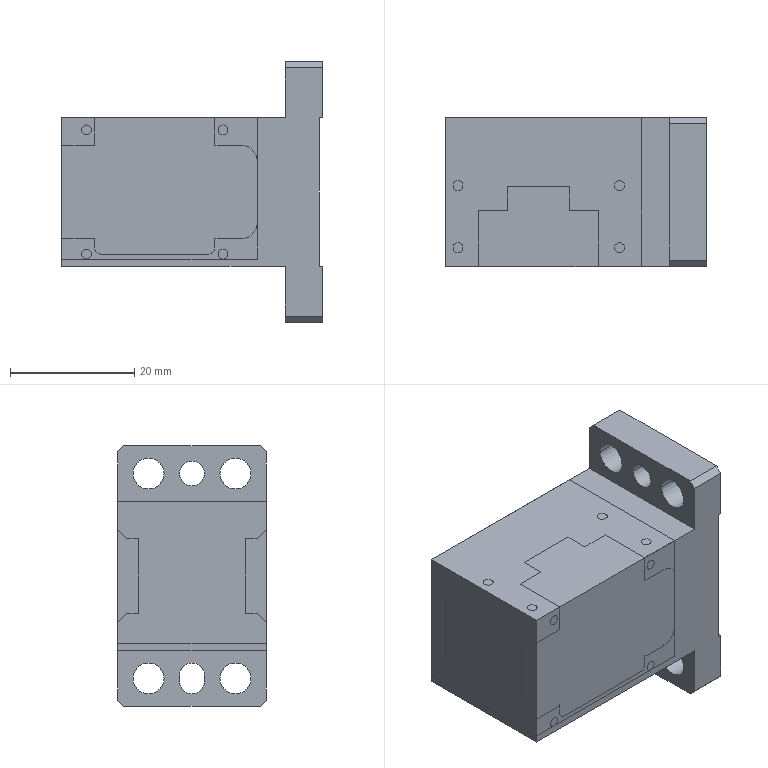NC program | NX | posted with a generic post | part box 42 x 24 x 42 mm
Lines 8998 to 10020 of 31406:
(CAVITY_MILL_COPY , TOOL : D2)
N17982 T02 M6
N17984 G54
N17986 G17 G0 G90 X-3.449 Y9.065 B0. C0. S6500 M3
N17988 G43 Z30. H2
N17990 Z0.465
N17992 G94 G1 Z-0.035 F1000.
N17994 G3 X-4.249 Y9.465 R1.
N17996 G1 X-5. F800.
N17998 G3 X-6.465 Y8. R1.465
N18000 G1 Y7.249
N18002 G3 X-6.065 Y6.449 R1.
N18004 G1 Z0.465
N18006 G0 X-3.414 Y9.03 Z0.43
N18008 G1 Z-0.07 F1000.
N18010 G3 X-4.214 Y9.43 R1.
N18012 G1 X-5. F800.
N18014 G3 X-6.43 Y8. R1.43
N18016 G1 Y7.214
N18018 G3 X-6.03 Y6.414 R1.
N18020 G1 Z0.43
N18022 G0 X-3.379 Y8.995 Z0.395
N18024 G1 Z-0.105 F1000.
N18026 G3 X-4.179 Y9.395 R1.
N18028 G1 X-5. F800.
N18030 G3 X-6.395 Y8. R1.395
N18032 G1 Y7.179
N18034 G3 X-5.995 Y6.379 R1.
N18036 G1 Z0.395
N18038 G0 X-3.344 Y8.96 Z0.36
N18040 G1 Z-0.14 F1000.
N18042 G3 X-4.144 Y9.36 R1.
N18044 G1 X-5. F800.
N18046 G3 X-6.36 Y8. R1.36
N18048 G1 Y7.144
N18050 G3 X-5.96 Y6.344 R1.
N18052 G1 Z0.36
N18054 G0 X-3.309 Y8.925 Z0.325
N18056 G1 Z-0.175 F1000.
N18058 G3 X-4.109 Y9.325 R1.
N18060 G1 X-5. F800.
N18062 G3 X-6.325 Y8. R1.325
N18064 G1 Y7.109
N18066 G3 X-5.925 Y6.309 R1.
N18068 G1 Z0.325
N18070 G0 X-3.274 Y8.89 Z0.29
N18072 G1 Z-0.21 F1000.
N18074 G3 X-4.074 Y9.29 R1.
N18076 G1 X-5. F800.
N18078 G3 X-6.29 Y8. R1.29
N18080 G1 Y7.074
N18082 G3 X-5.89 Y6.274 R1.
N18084 G1 Z0.29
N18086 G0 X-3.239 Y8.855 Z0.255
N18088 G1 Z-0.245 F1000.
N18090 G3 X-4.039 Y9.255 R1.
N18092 G1 X-5. F800.
N18094 G3 X-6.255 Y8. R1.255
N18096 G1 Y7.039
N18098 G3 X-5.855 Y6.239 R1.
N18100 G1 Z0.255
N18102 G0 X-3.204 Y8.82 Z0.22
N18104 G1 Z-0.28 F1000.
N18106 G3 X-4.004 Y9.22 R1.
N18108 G1 X-5. F800.
N18110 G3 X-6.22 Y8. R1.22
N18112 G1 Y7.004
N18114 G3 X-5.82 Y6.204 R1.
N18116 G1 Z0.22
N18118 G0 X-3.169 Y8.785 Z0.185
N18120 G1 Z-0.315 F1000.
N18122 G3 X-3.969 Y9.185 R1.
N18124 G1 X-5. F800.
N18126 G3 X-6.185 Y8. R1.185
N18128 G1 Y6.969
N18130 G3 X-5.785 Y6.169 R1.
N18132 G1 Z0.185
N18134 G0 X-3.134 Y8.75 Z0.15
N18136 G1 Z-0.35 F1000.
N18138 G3 X-3.934 Y9.15 R1.
N18140 G1 X-5. F800.
N18142 G3 X-6.15 Y8. R1.15
N18144 G1 Y6.934
N18146 G3 X-5.75 Y6.134 R1.
N18148 G1 Z0.15
N18150 G0 X-3.099 Y8.715 Z0.115
N18152 G1 Z-0.385 F1000.
N18154 G3 X-3.899 Y9.115 R1.
N18156 G1 X-5. F800.
N18158 G3 X-6.115 Y8. R1.115
N18160 G1 Y6.899
N18162 G3 X-5.715 Y6.099 R1.
N18164 G1 Z0.115
N18166 G0 X-3.064 Y8.68 Z0.08
N18168 G1 Z-0.42 F1000.
N18170 G3 X-3.864 Y9.08 R1.
N18172 G1 X-5. F800.
N18174 G3 X-6.08 Y8. R1.08
N18176 G1 Y6.864
N18178 G3 X-5.68 Y6.064 R1.
N18180 G1 Z0.08
N18182 G0 X-3.029 Y8.645 Z0.045
N18184 G1 Z-0.455 F1000.
N18186 G3 X-3.829 Y9.045 R1.
N18188 G1 X-5. F800.
N18190 G3 X-6.045 Y8. R1.045
N18192 G1 Y6.829
N18194 G3 X-5.645 Y6.029 R1.
N18196 G1 Z0.045
N18198 G0 X-2.994 Y8.61 Z0.01
N18200 G1 Z-0.49 F1000.
N18202 G3 X-3.794 Y9.01 R1.
N18204 G1 X-5. F800.
N18206 G3 X-6.01 Y8. R1.01
N18208 G1 Y6.794
N18210 G3 X-5.61 Y5.994 R1.
N18212 G1 Z0.01
N18214 G0 X-2.959 Y8.575 Z-0.025
N18216 G1 Z-0.525 F1000.
N18218 G3 X-3.759 Y8.975 R1.
N18220 G1 X-5. F800.
N18222 G3 X-5.975 Y8. R0.975
N18224 G1 Y6.759
N18226 G3 X-5.575 Y5.959 R1.
N18228 G1 Z-0.025
N18230 G0 X-2.924 Y8.54 Z-0.06
N18232 G1 Z-0.56 F1000.
N18234 G3 X-3.724 Y8.94 R1.
N18236 G1 X-5. F800.
N18238 G3 X-5.94 Y8. R0.94
N18240 G1 Y6.724
N18242 G3 X-5.54 Y5.924 R1.
N18244 G1 Z-0.06
N18246 G0 X-2.889 Y8.505 Z-0.095
N18248 G1 Z-0.595 F1000.
N18250 G3 X-3.689 Y8.905 R1.
N18252 G1 X-5. F800.
N18254 G3 X-5.905 Y8. R0.905
N18256 G1 Y6.689
N18258 G3 X-5.505 Y5.889 R1.
N18260 G1 Z-0.095
N18262 G0 X-2.854 Y8.47 Z-0.13
N18264 G1 Z-0.63 F1000.
N18266 G3 X-3.654 Y8.87 R1.
N18268 G1 X-5. F800.
N18270 G3 X-5.87 Y8. R0.87
N18272 G1 Y6.654
N18274 G3 X-5.47 Y5.854 R1.
N18276 G1 Z-0.13
N18278 G0 X-2.819 Y8.435 Z-0.165
N18280 G1 Z-0.665 F1000.
N18282 G3 X-3.619 Y8.835 R1.
N18284 G1 X-5. F800.
N18286 G3 X-5.835 Y8. R0.835
N18288 G1 Y6.619
N18290 G3 X-5.435 Y5.819 R1.
N18292 G1 Z-0.165
N18294 G0 X-2.784 Y8.4 Z-0.2
N18296 G1 Z-0.7 F1000.
N18298 G3 X-3.584 Y8.8 R1.
N18300 G1 X-5. F800.
N18302 G3 X-5.8 Y8. R0.8
N18304 G1 Y6.584
N18306 G3 X-5.4 Y5.784 R1.
N18308 G1 Z-0.2
N18310 G0 X-2.749 Y8.365 Z-0.235
N18312 G1 Z-0.735 F1000.
N18314 G3 X-3.549 Y8.765 R1.
N18316 G1 X-5. F800.
N18318 G3 X-5.765 Y8. R0.765
N18320 G1 Y6.549
N18322 G3 X-5.365 Y5.749 R1.
N18324 G1 Z-0.235
N18326 G0 X-2.714 Y8.33 Z-0.27
N18328 G1 Z-0.77 F1000.
N18330 G3 X-3.514 Y8.73 R1.
N18332 G1 X-5. F800.
N18334 G3 X-5.73 Y8. R0.73
N18336 G1 Y6.514
N18338 G3 X-5.33 Y5.714 R1.
N18340 G1 Z-0.27
N18342 G0 X-2.679 Y8.295 Z-0.305
N18344 G1 Z-0.805 F1000.
N18346 G3 X-3.479 Y8.695 R1.
N18348 G1 X-5. F800.
N18350 G3 X-5.695 Y8. R0.695
N18352 G1 Y6.479
N18354 G3 X-5.295 Y5.679 R1.
N18356 G1 Z-0.305
N18358 G0 X-2.644 Y8.26 Z-0.34
N18360 G1 Z-0.84 F1000.
N18362 G3 X-3.444 Y8.66 R1.
N18364 G1 X-5. F800.
N18366 G3 X-5.66 Y8. R0.66
N18368 G1 Y6.444
N18370 G3 X-5.26 Y5.644 R1.
N18372 G1 Z-0.34
N18374 G0 X-2.609 Y8.225 Z-0.375
N18376 G1 Z-0.875 F1000.
N18378 G3 X-3.409 Y8.625 R1.
N18380 G1 X-5. F800.
N18382 G3 X-5.625 Y8. R0.625
N18384 G1 Y6.409
N18386 G3 X-5.225 Y5.609 R1.
N18388 G1 Z-0.375
N18390 G0 X-2.574 Y8.19 Z-0.41
N18392 G1 Z-0.91 F1000.
N18394 G3 X-3.374 Y8.59 R1.
N18396 G1 X-5. F800.
N18398 G3 X-5.59 Y8. R0.59
N18400 G1 Y6.374
N18402 G3 X-5.19 Y5.574 R1.
N18404 G1 Z-0.41
N18406 G0 X-2.539 Y8.155 Z-0.445
N18408 G1 Z-0.945 F1000.
N18410 G3 X-3.339 Y8.555 R1.
N18412 G1 X-5. F800.
N18414 G3 X-5.555 Y8. R0.555
N18416 G1 Y6.339
N18418 G3 X-5.155 Y5.539 R1.
N18420 G1 Z-0.445
N18422 G0 X-2.504 Y8.12 Z-0.48
N18424 G1 Z-0.98 F1000.
N18426 G3 X-3.304 Y8.52 R1.
N18428 G1 X-5. F800.
N18430 G3 X-5.52 Y8. R0.52
N18432 G1 Y6.304
N18434 G3 X-5.12 Y5.504 R1.
N18436 G1 Z-0.48
N18438 G0 X-2.469 Y8.085 Z-0.515
N18440 G1 Z-1.015 F1000.
N18442 G3 X-3.269 Y8.485 R1.
N18444 G1 X-5. F800.
N18446 G3 X-5.485 Y8. R0.485
N18448 G1 Y6.269
N18450 G3 X-5.085 Y5.469 R1.
N18452 G1 Z-0.515
N18454 G0 X-2.434 Y8.05 Z-0.55
N18456 G1 Z-1.05 F1000.
N18458 G3 X-3.234 Y8.45 R1.
N18460 G1 X-5. F800.
N18462 G3 X-5.45 Y8. R0.45
N18464 G1 Y6.234
N18466 G3 X-5.05 Y5.434 R1.
N18468 G1 Z-0.55
N18470 G0 X-2.399 Y8.015 Z-0.585
N18472 G1 Z-1.085 F1000.
N18474 G3 X-3.199 Y8.415 R1.
N18476 G1 X-5. F800.
N18478 G3 X-5.415 Y8. R0.415
N18480 G1 Y6.199
N18482 G3 X-5.015 Y5.399 R1.
N18484 G1 Z-0.585
N18486 G0 X-2.364 Y7.98 Z-0.62
N18488 G1 Z-1.12 F1000.
N18490 G3 X-3.164 Y8.38 R1.
N18492 G1 X-5. F800.
N18494 G3 X-5.38 Y8. R0.38
N18496 G1 Y6.164
N18498 G3 X-4.98 Y5.364 R1.
N18500 G1 Z-0.62
N18502 G0 X-2.329 Y7.945 Z-0.655
N18504 G1 Z-1.155 F1000.
N18506 G3 X-3.129 Y8.345 R1.
N18508 G1 X-5. F800.
N18510 G3 X-5.345 Y8. R0.345
N18512 G1 Y6.129
N18514 G3 X-4.945 Y5.329 R1.
N18516 G1 Z-0.655
N18518 G0 X-2.294 Y7.91 Z-0.69
N18520 G1 Z-1.19 F1000.
N18522 G3 X-3.094 Y8.31 R1.
N18524 G1 X-5. F800.
N18526 G3 X-5.31 Y8. R0.31
N18528 G1 Y6.094
N18530 G3 X-4.91 Y5.294 R1.
N18532 G1 Z-0.69
N18534 G0 X-2.259 Y7.875 Z-0.725
N18536 G1 Z-1.225 F1000.
N18538 G3 X-3.059 Y8.275 R1.
N18540 G1 X-5. F800.
N18542 G3 X-5.275 Y8. R0.275
N18544 G1 Y6.059
N18546 G3 X-4.875 Y5.259 R1.
N18548 G1 Z-0.725
N18550 G0 X-2.224 Y7.84 Z-0.76
N18552 G1 Z-1.26 F1000.
N18554 G3 X-3.024 Y8.24 R1.
N18556 G1 X-5. F800.
N18558 G3 X-5.24 Y8. R0.24
N18560 G1 Y6.024
N18562 G3 X-4.84 Y5.224 R1.
N18564 G1 Z-0.76
N18566 G0 X-2.189 Y7.805 Z-0.795
N18568 G1 Z-1.295 F1000.
N18570 G3 X-2.989 Y8.205 R1.
N18572 G1 X-5. F800.
N18574 G3 X-5.205 Y8. R0.205
N18576 G1 Y5.989
N18578 G3 X-4.805 Y5.189 R1.
N18580 G1 Z-0.795
N18582 G0 X-2.154 Y7.77 Z-0.83
N18584 G1 Z-1.33 F1000.
N18586 G3 X-2.954 Y8.17 R1.
N18588 G1 X-5. F800.
N18590 G3 X-5.17 Y8. R0.17
N18592 G1 Y5.954
N18594 G3 X-4.77 Y5.154 R1.
N18596 G1 Z-0.83
N18598 G0 X-2.119 Y7.735 Z-0.865
N18600 G1 Z-1.365 F1000.
N18602 G3 X-2.919 Y8.135 R1.
N18604 G1 X-5. F800.
N18606 G3 X-5.135 Y8. R0.135
N18608 G1 Y5.919
N18610 G3 X-4.735 Y5.119 R1.
N18612 G1 Z-0.865
N18614 G0 X-2.084 Y7.7 Z-0.9
N18616 G1 Z-1.4 F1000.
N18618 G3 X-2.884 Y8.1 R1.
N18620 G1 X-5. F800.
N18622 X-5.055 Y8.095
N18624 X-5.095 Y8.055
N18626 X-5.1 Y8.
N18628 Y5.884
N18630 G3 X-4.7 Y5.084 R1.
N18632 G1 Z-0.9
N18634 G0 X-2.049 Y7.665 Z-0.935
N18636 G1 Z-1.435 F1000.
N18638 G3 X-2.849 Y8.065 R1.
N18640 G1 X-5. F800.
N18642 X-5.038
N18644 X-5.065 Y8.038
N18646 Y8.
N18648 Y5.849
N18650 G3 X-4.665 Y5.049 R1.
N18652 G1 Z-0.935
N18654 G0 X-2.014 Y7.63 Z-0.97
N18656 G1 Z-1.47 F1000.
N18658 G3 X-2.814 Y8.03 R1.
N18660 G1 X-5. F800.
N18662 X-5.02 Y8.035
N18664 X-5.035 Y8.02
N18666 X-5.03 Y8.
N18668 Y5.814
N18670 G3 X-4.63 Y5.014 R1.
N18672 G1 Z-0.97
N18674 G0 X-1.984 Y7.6 Z-1.005
N18676 G1 Z-1.505 F1000.
N18678 G3 X-2.784 Y8. R1.
N18680 G1 X-5. F800.
N18682 Y7.964
N18684 Y5.784
N18686 G3 X-4.6 Y4.984 R1.
N18688 G1 Z-1.005
N18690 G0 X-1.984 Y7.6 Z-1.04
N18692 G1 Z-1.54 F1000.
N18694 G3 X-2.784 Y8. R1.
N18696 G1 X-5. F800.
N18698 Y5.784
N18700 G3 X-4.6 Y4.984 R1.
N18702 G1 Z-1.04
N18704 G0 X-1.984 Y7.6 Z-1.075
N18706 G1 Z-1.575 F1000.
N18708 G3 X-2.784 Y8. R1.
N18710 G1 X-5. F800.
N18712 Y5.784
N18714 G3 X-4.6 Y4.984 R1.
N18716 G1 Z-1.075
N18718 G0 X-1.984 Y7.6 Z-1.11
N18720 G1 Z-1.61 F1000.
N18722 G3 X-2.784 Y8. R1.
N18724 G1 X-5. F800.
N18726 Y5.784
N18728 G3 X-4.6 Y4.984 R1.
N18730 G1 Z-1.11
N18732 G0 X-1.984 Y7.6 Z-1.145
N18734 G1 Z-1.645 F1000.
N18736 G3 X-2.784 Y8. R1.
N18738 G1 X-5. F800.
N18740 Y5.784
N18742 G3 X-4.6 Y4.984 R1.
N18744 G1 Z-1.145
N18746 G0 X-1.984 Y7.6 Z-1.18
N18748 G1 Z-1.68 F1000.
N18750 G3 X-2.784 Y8. R1.
N18752 G1 X-5. F800.
N18754 Y5.784
N18756 G3 X-4.6 Y4.984 R1.
N18758 G1 Z-1.18
N18760 G0 X-1.984 Y7.6 Z-1.215
N18762 G1 Z-1.715 F1000.
N18764 G3 X-2.784 Y8. R1.
N18766 G1 X-5. F800.
N18768 Y5.784
N18770 G3 X-4.6 Y4.984 R1.
N18772 G1 Z-1.215
N18774 G0 X-1.984 Y7.6 Z-1.25
N18776 G1 Z-1.75 F1000.
N18778 G3 X-2.784 Y8. R1.
N18780 G1 X-5. F800.
N18782 Y5.784
N18784 G3 X-4.6 Y4.984 R1.
N18786 G1 Z-1.25
N18788 G0 X-1.984 Y7.6 Z-1.285
N18790 G1 Z-1.785 F1000.
N18792 G3 X-2.784 Y8. R1.
N18794 G1 X-5. F800.
N18796 Y5.784
N18798 G3 X-4.6 Y4.984 R1.
N18800 G1 Z-1.285
N18802 G0 X-1.984 Y7.6 Z-1.32
N18804 G1 Z-1.82 F1000.
N18806 G3 X-2.784 Y8. R1.
N18808 G1 X-5. F800.
N18810 Y5.784
N18812 G3 X-4.6 Y4.984 R1.
N18814 G1 Z-1.32
N18816 G0 X-1.984 Y7.6 Z-1.355
N18818 G1 Z-1.855 F1000.
N18820 G3 X-2.784 Y8. R1.
N18822 G1 X-5. F800.
N18824 Y5.784
N18826 G3 X-4.6 Y4.984 R1.
N18828 G1 Z-1.355
N18830 G0 X-1.984 Y7.6 Z-1.39
N18832 G1 Z-1.89 F1000.
N18834 G3 X-2.784 Y8. R1.
N18836 G1 X-5. F800.
N18838 Y5.784
N18840 G3 X-4.6 Y4.984 R1.
N18842 G1 Z-1.39
N18844 G0 X-1.984 Y7.6 Z-1.425
N18846 G1 Z-1.925 F1000.
N18848 G3 X-2.784 Y8. R1.
N18850 G1 X-5. F800.
N18852 Y5.784
N18854 G3 X-4.6 Y4.984 R1.
N18856 G1 Z-1.425
N18858 G0 X-1.984 Y7.6 Z-1.46
N18860 G1 Z-1.96 F1000.
N18862 G3 X-2.784 Y8. R1.
N18864 G1 X-5. F800.
N18866 Y5.784
N18868 G3 X-4.6 Y4.984 R1.
N18870 G1 Z-1.46
N18872 G0 X-1.984 Y7.6 Z-1.495
N18874 G1 Z-1.995 F1000.
N18876 G3 X-2.784 Y8. R1.
N18878 G1 X-5. F800.
N18880 Y5.784
N18882 G3 X-4.6 Y4.984 R1.
N18884 G1 Z-1.495
N18886 G0 X-1.984 Y7.6 Z-1.53
N18888 G1 Z-2.03 F1000.
N18890 G3 X-2.784 Y8. R1.
N18892 G1 X-5. F800.
N18894 Y5.784
N18896 G3 X-4.6 Y4.984 R1.
N18898 G1 Z-1.53
N18900 G0 X-1.984 Y7.6 Z-1.565
N18902 G1 Z-2.065 F1000.
N18904 G3 X-2.784 Y8. R1.
N18906 G1 X-5. F800.
N18908 Y5.784
N18910 G3 X-4.6 Y4.984 R1.
N18912 G1 Z-1.565
N18914 G0 X-1.984 Y7.6 Z-1.6
N18916 G1 Z-2.1 F1000.
N18918 G3 X-2.784 Y8. R1.
N18920 G1 X-5. F800.
N18922 Y5.784
N18924 G3 X-4.6 Y4.984 R1.
N18926 G1 Z-1.6
N18928 G0 X-1.984 Y7.6 Z-1.635
N18930 G1 Z-2.135 F1000.
N18932 G3 X-2.784 Y8. R1.
N18934 G1 X-5. F800.
N18936 Y5.784
N18938 G3 X-4.6 Y4.984 R1.
N18940 G1 Z-1.635
N18942 G0 X-1.984 Y7.6 Z-1.67
N18944 G1 Z-2.17 F1000.
N18946 G3 X-2.784 Y8. R1.
N18948 G1 X-5. F800.
N18950 Y5.784
N18952 G3 X-4.6 Y4.984 R1.
N18954 G1 Z-1.67
N18956 G0 X-1.984 Y7.6 Z-1.705
N18958 G1 Z-2.205 F1000.
N18960 G3 X-2.784 Y8. R1.
N18962 G1 X-5. F800.
N18964 Y5.784
N18966 G3 X-4.6 Y4.984 R1.
N18968 G1 Z-1.705
N18970 G0 X-1.984 Y7.6 Z-1.74
N18972 G1 Z-2.24 F1000.
N18974 G3 X-2.784 Y8. R1.
N18976 G1 X-5. F800.
N18978 Y5.784
N18980 G3 X-4.6 Y4.984 R1.
N18982 G1 Z-1.74
N18984 G0 X-1.984 Y7.6 Z-1.775
N18986 G1 Z-2.275 F1000.
N18988 G3 X-2.784 Y8. R1.
N18990 G1 X-5. F800.
N18992 Y5.784
N18994 G3 X-4.6 Y4.984 R1.
N18996 G1 Z-1.775
N18998 G0 X-1.984 Y7.6 Z-1.81
N19000 G1 Z-2.31 F1000.
N19002 G3 X-2.784 Y8. R1.
N19004 G1 X-5. F800.
N19006 Y5.784
N19008 G3 X-4.6 Y4.984 R1.
N19010 G1 Z-1.81
N19012 G0 X-1.984 Y7.6 Z-1.845
N19014 G1 Z-2.345 F1000.
N19016 G3 X-2.784 Y8. R1.
N19018 G1 X-5. F800.
N19020 Y5.784
N19022 G3 X-4.6 Y4.984 R1.
N19024 G1 Z-1.845
N19026 G0 X-1.984 Y7.6 Z-1.88
N19028 G1 Z-2.38 F1000.
N19030 G3 X-2.784 Y8. R1.
N19032 G1 X-5. F800.
N19034 Y5.784
N19036 G3 X-4.6 Y4.984 R1.
N19038 G1 Z-1.88
N19040 G0 X-1.984 Y7.6 Z-1.915
N19042 G1 Z-2.415 F1000.
N19044 G3 X-2.784 Y8. R1.
N19046 G1 X-5. F800.
N19048 Y5.784
N19050 G3 X-4.6 Y4.984 R1.
N19052 G1 Z-1.915
N19054 G0 X-1.984 Y7.6 Z-1.95
N19056 G1 Z-2.45 F1000.
N19058 G3 X-2.784 Y8. R1.
N19060 G1 X-5. F800.
N19062 Y5.784
N19064 G3 X-4.6 Y4.984 R1.
N19066 G1 Z-1.95
N19068 G0 X-1.984 Y7.6 Z-1.985
N19070 G1 Z-2.485 F1000.
N19072 G3 X-2.784 Y8. R1.
N19074 G1 X-5. F800.
N19076 Y5.784
N19078 G3 X-4.6 Y4.984 R1.
N19080 G1 Z-1.985
N19082 G0 X-1.984 Y7.6 Z-2.02
N19084 G1 Z-2.52 F1000.
N19086 G3 X-2.784 Y8. R1.
N19088 G1 X-5. F800.
N19090 Y5.784
N19092 G3 X-4.6 Y4.984 R1.
N19094 G1 Z-2.02
N19096 G0 X-1.984 Y7.6 Z-2.055
N19098 G1 Z-2.555 F1000.
N19100 G3 X-2.784 Y8. R1.
N19102 G1 X-5. F800.
N19104 Y5.784
N19106 G3 X-4.6 Y4.984 R1.
N19108 G1 Z-2.055
N19110 G0 X-1.984 Y7.6 Z-2.09
N19112 G1 Z-2.59 F1000.
N19114 G3 X-2.784 Y8. R1.
N19116 G1 X-5. F800.
N19118 Y5.784
N19120 G3 X-4.6 Y4.984 R1.
N19122 G1 Z-2.09
N19124 G0 X-1.984 Y7.6 Z-2.125
N19126 G1 Z-2.625 F1000.
N19128 G3 X-2.784 Y8. R1.
N19130 G1 X-5. F800.
N19132 Y5.784
N19134 G3 X-4.6 Y4.984 R1.
N19136 G1 Z-2.125
N19138 G0 X-1.984 Y7.6 Z-2.16
N19140 G1 Z-2.66 F1000.
N19142 G3 X-2.784 Y8. R1.
N19144 G1 X-5. F800.
N19146 Y5.784
N19148 G3 X-4.6 Y4.984 R1.
N19150 G1 Z-2.16
N19152 G0 X-1.984 Y7.6 Z-2.195
N19154 G1 Z-2.695 F1000.
N19156 G3 X-2.784 Y8. R1.
N19158 G1 X-5. F800.
N19160 Y5.784
N19162 G3 X-4.6 Y4.984 R1.
N19164 G1 Z-2.195
N19166 G0 X-1.984 Y7.6 Z-2.23
N19168 G1 Z-2.73 F1000.
N19170 G3 X-2.784 Y8. R1.
N19172 G1 X-5. F800.
N19174 Y5.784
N19176 G3 X-4.6 Y4.984 R1.
N19178 G1 Z-2.23
N19180 G0 X-1.984 Y7.6 Z-2.265
N19182 G1 Z-2.765 F1000.
N19184 G3 X-2.784 Y8. R1.
N19186 G1 X-5. F800.
N19188 Y5.784
N19190 G3 X-4.6 Y4.984 R1.
N19192 G1 Z-2.265
N19194 G0 X-1.984 Y7.6 Z-2.3
N19196 G1 Z-2.8 F1000.
N19198 G3 X-2.784 Y8. R1.
N19200 G1 X-5. F800.
N19202 Y5.784
N19204 G3 X-4.6 Y4.984 R1.
N19206 G1 Z-2.3
N19208 G0 X-1.984 Y7.6 Z-2.335
N19210 G1 Z-2.835 F1000.
N19212 G3 X-2.784 Y8. R1.
N19214 G1 X-5. F800.
N19216 Y5.784
N19218 G3 X-4.6 Y4.984 R1.
N19220 G1 Z-2.335
N19222 G0 X-1.984 Y7.6 Z-2.37
N19224 G1 Z-2.87 F1000.
N19226 G3 X-2.784 Y8. R1.
N19228 G1 X-5. F800.
N19230 Y5.784
N19232 G3 X-4.6 Y4.984 R1.
N19234 G1 Z-2.37
N19236 G0 X-1.984 Y7.6 Z-2.405
N19238 G1 Z-2.905 F1000.
N19240 G3 X-2.784 Y8. R1.
N19242 G1 X-5. F800.
N19244 Y5.784
N19246 G3 X-4.6 Y4.984 R1.
N19248 G1 Z-2.405
N19250 G0 X-1.984 Y7.6 Z-2.44
N19252 G1 Z-2.94 F1000.
N19254 G3 X-2.784 Y8. R1.
N19256 G1 X-5. F800.
N19258 Y5.784
N19260 G3 X-4.6 Y4.984 R1.
N19262 G1 Z-2.44
N19264 G0 X-1.984 Y7.6 Z-2.475
N19266 G1 Z-2.975 F1000.
N19268 G3 X-2.784 Y8. R1.
N19270 G1 X-5. F800.
N19272 Y5.784
N19274 G3 X-4.6 Y4.984 R1.
N19276 G1 Z-2.475
N19278 G0 X-1.984 Y7.6 Z-2.51
N19280 G1 Z-3.01 F1000.
N19282 G3 X-2.784 Y8. R1.
N19284 G1 X-5. F800.
N19286 Y5.784
N19288 G3 X-4.6 Y4.984 R1.
N19290 G1 Z-2.51
N19292 G0 X-1.984 Y7.6 Z-2.545
N19294 G1 Z-3.045 F1000.
N19296 G3 X-2.784 Y8. R1.
N19298 G1 X-5. F800.
N19300 Y5.784
N19302 G3 X-4.6 Y4.984 R1.
N19304 G1 Z-2.545
N19306 G0 X-1.984 Y7.6 Z-2.58
N19308 G1 Z-3.08 F1000.
N19310 G3 X-2.784 Y8. R1.
N19312 G1 X-5. F800.
N19314 Y5.784
N19316 G3 X-4.6 Y4.984 R1.
N19318 G1 Z-2.58
N19320 G0 X-1.984 Y7.6 Z-2.615
N19322 G1 Z-3.115 F1000.
N19324 G3 X-2.784 Y8. R1.
N19326 G1 X-5. F800.
N19328 Y5.784
N19330 G3 X-4.6 Y4.984 R1.
N19332 G1 Z-2.615
N19334 G0 X-1.984 Y7.6 Z-2.65
N19336 G1 Z-3.15 F1000.
N19338 G3 X-2.784 Y8. R1.
N19340 G1 X-5. F800.
N19342 Y5.784
N19344 G3 X-4.6 Y4.984 R1.
N19346 G1 Z-2.65
N19348 G0 X-1.984 Y7.6 Z-2.685
N19350 G1 Z-3.185 F1000.
N19352 G3 X-2.784 Y8. R1.
N19354 G1 X-5. F800.
N19356 Y5.784
N19358 G3 X-4.6 Y4.984 R1.
N19360 G1 Z-2.685
N19362 G0 X-1.984 Y7.6 Z-2.72
N19364 G1 Z-3.22 F1000.
N19366 G3 X-2.784 Y8. R1.
N19368 G1 X-5. F800.
N19370 Y5.784
N19372 G3 X-4.6 Y4.984 R1.
N19374 G1 Z-2.72
N19376 G0 X-1.984 Y7.6 Z-2.755
N19378 G1 Z-3.255 F1000.
N19380 G3 X-2.784 Y8. R1.
N19382 G1 X-5. F800.
N19384 Y5.784
N19386 G3 X-4.6 Y4.984 R1.
N19388 G1 Z-2.755
N19390 G0 X-1.984 Y7.6 Z-2.79
N19392 G1 Z-3.29 F1000.
N19394 G3 X-2.784 Y8. R1.
N19396 G1 X-5. F800.
N19398 Y5.784
N19400 G3 X-4.6 Y4.984 R1.
N19402 G1 Z-2.79
N19404 G0 X-1.984 Y7.6 Z-2.825
N19406 G1 Z-3.325 F1000.
N19408 G3 X-2.784 Y8. R1.
N19410 G1 X-5. F800.
N19412 Y5.784
N19414 G3 X-4.6 Y4.984 R1.
N19416 G1 Z-2.825
N19418 G0 X-1.984 Y7.6 Z-2.86
N19420 G1 Z-3.36 F1000.
N19422 G3 X-2.784 Y8. R1.
N19424 G1 X-5. F800.
N19426 Y5.784
N19428 G3 X-4.6 Y4.984 R1.
N19430 G1 Z-2.86
N19432 G0 X-1.984 Y7.6 Z-2.895
N19434 G1 Z-3.395 F1000.
N19436 G3 X-2.784 Y8. R1.
N19438 G1 X-5. F800.
N19440 Y5.784
N19442 G3 X-4.6 Y4.984 R1.
N19444 G1 Z-2.895
N19446 G0 X-1.984 Y7.6 Z-2.93
N19448 G1 Z-3.43 F1000.
N19450 G3 X-2.784 Y8. R1.
N19452 G1 X-5. F800.
N19454 Y5.784
N19456 G3 X-4.6 Y4.984 R1.
N19458 G1 Z-2.93
N19460 G0 X-1.984 Y5.6 Z-2.965
N19462 G1 Z-3.465 F1000.
N19464 G3 X-2.784 Y6. R1.
N19466 G1 X-5. F800.
N19468 Y3.784
N19470 G3 X-4.733 Y3.104 R1.
N19472 G1 Z-2.965
N19474 G0 X-1.984 Y5.6 Z-3.
N19476 G1 Z-3.5 F1000.
N19478 G3 X-2.784 Y6. R1.
N19480 G1 X-5. F800.
N19482 Y3.784
N19484 G3 X-4.733 Y3.104 R1.
N19486 G1 Z-3.
N19488 G0 X-1.984 Y5.6 Z-3.034
N19490 G1 Z-3.534 F1000.
N19492 G3 X-2.784 Y6. R1.
N19494 G1 X-5. F800.
N19496 Y3.784
N19498 G3 X-4.733 Y3.104 R1.
N19500 G1 Z-3.034
N19502 G0 X-1.984 Y5.6 Z-3.069
N19504 G1 Z-3.569 F1000.
N19506 G3 X-2.784 Y6. R1.
N19508 G1 X-5. F800.
N19510 Y3.784
N19512 G3 X-4.733 Y3.104 R1.
N19514 G1 Z-3.069
N19516 G0 X-1.984 Y5.6 Z-3.104
N19518 G1 Z-3.604 F1000.
N19520 G3 X-2.784 Y6. R1.
N19522 G1 X-5. F800.
N19524 Y3.784
N19526 G3 X-4.733 Y3.104 R1.
N19528 G1 Z-3.104
N19530 G0 X-1.984 Y5.6 Z-3.139
N19532 G1 Z-3.639 F1000.
N19534 G3 X-2.784 Y6. R1.
N19536 G1 X-5. F800.
N19538 Y3.784
N19540 G3 X-4.733 Y3.104 R1.
N19542 G1 Z-3.139
N19544 G0 X-1.984 Y5.6 Z-3.174
N19546 G1 Z-3.674 F1000.
N19548 G3 X-2.784 Y6. R1.
N19550 G1 X-5. F800.
N19552 Y3.784
N19554 G3 X-4.733 Y3.104 R1.
N19556 G1 Z-3.174
N19558 G0 X-1.984 Y5.6 Z-3.209
N19560 G1 Z-3.709 F1000.
N19562 G3 X-2.784 Y6. R1.
N19564 G1 X-5. F800.
N19566 Y3.784
N19568 G3 X-4.733 Y3.104 R1.
N19570 G1 Z-3.209
N19572 G0 X-1.984 Y5.6 Z-3.243
N19574 G1 Z-3.743 F1000.
N19576 G3 X-2.784 Y6. R1.
N19578 G1 X-5. F800.
N19580 Y3.784
N19582 G3 X-4.733 Y3.104 R1.
N19584 G1 Z-3.243
N19586 G0 X-1.984 Y5.6 Z-3.278
N19588 G1 Z-3.778 F1000.
N19590 G3 X-2.784 Y6. R1.
N19592 G1 X-5. F800.
N19594 Y3.784
N19596 G3 X-4.733 Y3.104 R1.
N19598 G1 Z-3.278
N19600 G0 X-1.984 Y5.6 Z-3.313
N19602 G1 Z-3.813 F1000.
N19604 G3 X-2.784 Y6. R1.
N19606 G1 X-5. F800.
N19608 Y3.784
N19610 G3 X-4.733 Y3.104 R1.
N19612 G1 Z-3.313
N19614 G0 X-1.984 Y5.6 Z-3.348
N19616 G1 Z-3.848 F1000.
N19618 G3 X-2.784 Y6. R1.
N19620 G1 X-5. F800.
N19622 Y3.784
N19624 G3 X-4.733 Y3.104 R1.
N19626 G1 Z-3.348
N19628 G0 X-1.984 Y5.6 Z-3.383
N19630 G1 Z-3.883 F1000.
N19632 G3 X-2.784 Y6. R1.
N19634 G1 X-5. F800.
N19636 Y3.784
N19638 G3 X-4.733 Y3.104 R1.
N19640 G1 Z-3.383
N19642 G0 X-1.984 Y5.6 Z-3.417
N19644 G1 Z-3.917 F1000.
N19646 G3 X-2.784 Y6. R1.
N19648 G1 X-5. F800.
N19650 Y3.784
N19652 G3 X-4.733 Y3.104 R1.
N19654 G1 Z-3.417
N19656 G0 X-1.984 Y5.6 Z-3.452
N19658 G1 Z-3.952 F1000.
N19660 G3 X-2.784 Y6. R1.
N19662 G1 X-5. F800.
N19664 Y3.784
N19666 G3 X-4.733 Y3.104 R1.
N19668 G1 Z-3.452
N19670 G0 X-1.984 Y5.6 Z-3.487
N19672 G1 Z-3.987 F1000.
N19674 G3 X-2.784 Y6. R1.
N19676 G1 X-5. F800.
N19678 Y3.784
N19680 G3 X-4.733 Y3.104 R1.
N19682 G1 Z-3.487
N19684 G0 X-1.984 Y5.6 Z-3.522
N19686 G1 Z-4.022 F1000.
N19688 G3 X-2.784 Y6. R1.
N19690 G1 X-5. F800.
N19692 Y3.784
N19694 G3 X-4.733 Y3.104 R1.
N19696 G1 Z-3.522
N19698 G0 X-1.984 Y5.6 Z-3.557
N19700 G1 Z-4.057 F1000.
N19702 G3 X-2.784 Y6. R1.
N19704 G1 X-5. F800.
N19706 Y3.784
N19708 G3 X-4.733 Y3.104 R1.
N19710 G1 Z-3.557
N19712 G0 X-1.984 Y5.6 Z-3.591
N19714 G1 Z-4.091 F1000.
N19716 G3 X-2.784 Y6. R1.
N19718 G1 X-5. F800.
N19720 Y3.784
N19722 G3 X-4.733 Y3.104 R1.
N19724 G1 Z-3.591
N19726 G0 X-1.984 Y5.6 Z-3.626
N19728 G1 Z-4.126 F1000.
N19730 G3 X-2.784 Y6. R1.
N19732 G1 X-5. F800.
N19734 Y3.784
N19736 G3 X-4.733 Y3.104 R1.
N19738 G1 Z-3.626
N19740 G0 X-1.984 Y5.6 Z-3.661
N19742 G1 Z-4.161 F1000.
N19744 G3 X-2.784 Y6. R1.
N19746 G1 X-5. F800.
N19748 Y3.784
N19750 G3 X-4.733 Y3.104 R1.
N19752 G1 Z-3.661
N19754 G0 X-1.984 Y5.6 Z-3.696
N19756 G1 Z-4.196 F1000.
N19758 G3 X-2.784 Y6. R1.
N19760 G1 X-5. F800.
N19762 Y3.784
N19764 G3 X-4.733 Y3.104 R1.
N19766 G1 Z-3.696
N19768 G0 X-1.984 Y5.6 Z-3.731
N19770 G1 Z-4.231 F1000.
N19772 G3 X-2.784 Y6. R1.
N19774 G1 X-5. F800.
N19776 Y3.784
N19778 G3 X-4.733 Y3.104 R1.
N19780 G1 Z-3.731
N19782 G0 X-1.984 Y5.6 Z-3.766
N19784 G1 Z-4.266 F1000.
N19786 G3 X-2.784 Y6. R1.
N19788 G1 X-5. F800.
N19790 Y3.784
N19792 G3 X-4.733 Y3.104 R1.
N19794 G1 Z-3.766
N19796 G0 X-1.984 Y5.6 Z-3.8
N19798 G1 Z-4.3 F1000.
N19800 G3 X-2.784 Y6. R1.
N19802 G1 X-5. F800.
N19804 Y3.784
N19806 G3 X-4.733 Y3.104 R1.
N19808 G1 Z-3.8
N19810 G0 X-1.984 Y5.6 Z-3.835
N19812 G1 Z-4.335 F1000.
N19814 G3 X-2.784 Y6. R1.
N19816 G1 X-5. F800.
N19818 Y3.784
N19820 G3 X-4.733 Y3.104 R1.
N19822 G1 Z-3.835
N19824 G0 X-1.984 Y5.6 Z-3.87
N19826 G1 Z-4.37 F1000.
N19828 G3 X-2.784 Y6. R1.
N19830 G1 X-5. F800.
N19832 Y3.784
N19834 G3 X-4.733 Y3.104 R1.
N19836 G1 Z-3.87
N19838 G0 X-1.984 Y5.6 Z-3.905
N19840 G1 Z-4.405 F1000.
N19842 G3 X-2.784 Y6. R1.
N19844 G1 X-5. F800.
N19846 Y3.784
N19848 G3 X-4.733 Y3.104 R1.
N19850 G1 Z-3.905
N19852 G0 X-1.984 Y5.6 Z-3.94
N19854 G1 Z-4.44 F1000.
N19856 G3 X-2.784 Y6. R1.
N19858 G1 X-5. F800.
N19860 Y3.784
N19862 G3 X-4.733 Y3.104 R1.
N19864 G1 Z-3.94
N19866 G0 X-1.984 Y5.6 Z-3.974
N19868 G1 Z-4.474 F1000.
N19870 G3 X-2.784 Y6. R1.
N19872 G1 X-5. F800.
N19874 Y3.784
N19876 G3 X-4.733 Y3.104 R1.
N19878 G1 Z-3.974
N19880 G0 X-1.984 Y5.6 Z-4.009
N19882 G1 Z-4.509 F1000.
N19884 G3 X-2.784 Y6. R1.
N19886 G1 X-5. F800.
N19888 Y3.784
N19890 G3 X-4.733 Y3.104 R1.
N19892 G1 Z-4.009
N19894 G0 X-1.984 Y5.6 Z-4.044
N19896 G1 Z-4.544 F1000.
N19898 G3 X-2.784 Y6. R1.
N19900 G1 X-5. F800.
N19902 Y3.784
N19904 G3 X-4.733 Y3.104 R1.
N19906 G1 Z-4.044
N19908 G0 X-1.984 Y5.6 Z-4.079
N19910 G1 Z-4.579 F1000.
N19912 G3 X-2.784 Y6. R1.
N19914 G1 X-5. F800.
N19916 Y3.784
N19918 G3 X-4.733 Y3.104 R1.
N19920 G1 Z-4.079
N19922 G0 X-1.984 Y5.6 Z-4.114
N19924 G1 Z-4.614 F1000.
N19926 G3 X-2.784 Y6. R1.
N19928 G1 X-5. F800.
N19930 Y3.784
N19932 G3 X-4.733 Y3.104 R1.
N19934 G1 Z-4.114
N19936 G0 X-1.984 Y5.6 Z-4.148
N19938 G1 Z-4.648 F1000.
N19940 G3 X-2.784 Y6. R1.
N19942 G1 X-5. F800.
N19944 Y3.784
N19946 G3 X-4.733 Y3.104 R1.
N19948 G1 Z-4.148
N19950 G0 X-1.984 Y5.6 Z-4.183
N19952 G1 Z-4.683 F1000.
N19954 G3 X-2.784 Y6. R1.
N19956 G1 X-5. F800.
N19958 Y3.784
N19960 G3 X-4.733 Y3.104 R1.
N19962 G1 Z-4.183
N19964 G0 X-1.984 Y5.6 Z-4.218
N19966 G1 Z-4.718 F1000.
N19968 G3 X-2.784 Y6. R1.
N19970 G1 X-5. F800.
N19972 Y3.784
N19974 G3 X-4.733 Y3.104 R1.
N19976 G1 Z-4.218
N19978 G0 X-1.984 Y5.6 Z-4.253
N19980 G1 Z-4.753 F1000.
N19982 G3 X-2.784 Y6. R1.
N19984 G1 X-5. F800.
N19986 Y3.784
N19988 G3 X-4.733 Y3.104 R1.
N19990 G1 Z-4.253
N19992 G0 X-1.984 Y5.6 Z-4.288
N19994 G1 Z-4.788 F1000.
N19996 G3 X-2.784 Y6. R1.
N19998 G1 X-5. F800.
N20000 Y3.784
N20002 G3 X-4.733 Y3.104 R1.
N20004 G1 Z-4.288
N20006 G0 X-1.984 Y5.6 Z-4.323
N20008 G1 Z-4.823 F1000.
N20010 G3 X-2.784 Y6. R1.
N20012 G1 X-5. F800.
N20014 Y3.784
N20016 G3 X-4.733 Y3.104 R1.
N20018 G1 Z-4.323
N20020 G0 X-1.984 Y5.6 Z-4.357